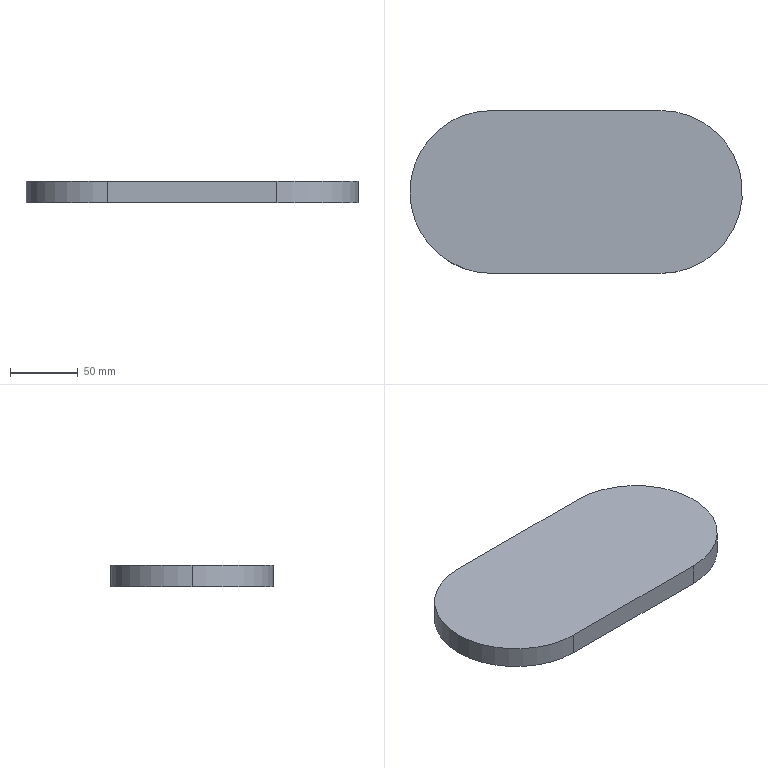Part | SolidWorks | features Extrusion 1 | 1 solid | 7 faces | box 245 x 120 x 16 mm | volume 420956 mm3 | plane 4 | cylinder 3 | commonest cylinder face diameters 120 x3
STEP:
#1=CARTESIAN_POINT('',(-122.5,0.,16.));
#2=VERTEX_POINT('',#1);
#3=CARTESIAN_POINT('',(-62.5,-60.,16.));
#4=VERTEX_POINT('',#3);
#5=CARTESIAN_POINT('',(-62.5,0.,16.));
#6=DIRECTION('',(0.,0.,1.));
#7=DIRECTION('',(1.,0.,0.));
#8=AXIS2_PLACEMENT_3D('',#5,#6,#7);
#9=CIRCLE('',#8,60.);
#10=EDGE_CURVE('',#2,#4,#9,.T.);
#11=ORIENTED_EDGE('',*,*,#10,.F.);
#12=CARTESIAN_POINT('',(-122.5,0.,0.));
#13=VERTEX_POINT('',#12);
#14=CARTESIAN_POINT('',(-122.5,0.,16.));
#15=DIRECTION('',(0.,0.,-1.));
#16=VECTOR('',#15,1000.);
#17=LINE('',#14,#16);
#18=EDGE_CURVE('',#2,#13,#17,.T.);
#19=ORIENTED_EDGE('',*,*,#18,.T.);
#20=CARTESIAN_POINT('',(-62.5,-60.,0.));
#21=VERTEX_POINT('',#20);
#22=CARTESIAN_POINT('',(-62.5,0.,0.));
#23=DIRECTION('',(0.,0.,1.));
#24=DIRECTION('',(1.,0.,0.));
#25=AXIS2_PLACEMENT_3D('',#22,#23,#24);
#26=CIRCLE('',#25,60.);
#27=EDGE_CURVE('',#13,#21,#26,.T.);
#28=ORIENTED_EDGE('',*,*,#27,.T.);
#29=CARTESIAN_POINT('',(-62.5,-60.,16.));
#30=DIRECTION('',(0.,0.,-1.));
#31=VECTOR('',#30,1000.);
#32=LINE('',#29,#31);
#33=EDGE_CURVE('',#4,#21,#32,.T.);
#34=ORIENTED_EDGE('',*,*,#33,.F.);
#35=EDGE_LOOP('',(#11,#19,#28,#34));
#36=FACE_OUTER_BOUND('',#35,.T.);
#37=CARTESIAN_POINT('',(-62.5,0.,16.));
#38=DIRECTION('',(0.,0.,-1.));
#39=DIRECTION('',(-1.,0.,0.));
#40=AXIS2_PLACEMENT_3D('',#37,#38,#39);
#41=CYLINDRICAL_SURFACE('',#40,60.);
#42=ADVANCED_FACE('',(#36),#41,.T.);
#43=ORIENTED_EDGE('',*,*,#18,.F.);
#44=CARTESIAN_POINT('',(-62.5,60.,16.));
#45=VERTEX_POINT('',#44);
#46=CARTESIAN_POINT('',(-62.5,0.,16.));
#47=DIRECTION('',(0.,0.,1.));
#48=DIRECTION('',(1.,0.,0.));
#49=AXIS2_PLACEMENT_3D('',#46,#47,#48);
#50=CIRCLE('',#49,60.);
#51=EDGE_CURVE('',#45,#2,#50,.T.);
#52=ORIENTED_EDGE('',*,*,#51,.F.);
#53=CARTESIAN_POINT('',(-62.5,60.,0.));
#54=VERTEX_POINT('',#53);
#55=CARTESIAN_POINT('',(-62.5,60.,16.));
#56=DIRECTION('',(0.,0.,-1.));
#57=VECTOR('',#56,1000.);
#58=LINE('',#55,#57);
#59=EDGE_CURVE('',#45,#54,#58,.T.);
#60=ORIENTED_EDGE('',*,*,#59,.T.);
#61=CARTESIAN_POINT('',(-62.5,0.,0.));
#62=DIRECTION('',(0.,0.,1.));
#63=DIRECTION('',(1.,0.,0.));
#64=AXIS2_PLACEMENT_3D('',#61,#62,#63);
#65=CIRCLE('',#64,60.);
#66=EDGE_CURVE('',#54,#13,#65,.T.);
#67=ORIENTED_EDGE('',*,*,#66,.T.);
#68=EDGE_LOOP('',(#43,#52,#60,#67));
#69=FACE_OUTER_BOUND('',#68,.T.);
#70=CARTESIAN_POINT('',(-62.5,0.,16.));
#71=DIRECTION('',(0.,0.,-1.));
#72=DIRECTION('',(-1.,0.,0.));
#73=AXIS2_PLACEMENT_3D('',#70,#71,#72);
#74=CYLINDRICAL_SURFACE('',#73,60.);
#75=ADVANCED_FACE('',(#69),#74,.T.);
#76=CARTESIAN_POINT('',(62.5,-60.,0.));
#77=VERTEX_POINT('',#76);
#78=CARTESIAN_POINT('',(-62.5,-60.,0.));
#79=DIRECTION('',(1.,0.,0.));
#80=VECTOR('',#79,1000.);
#81=LINE('',#78,#80);
#82=EDGE_CURVE('',#21,#77,#81,.T.);
#83=ORIENTED_EDGE('',*,*,#82,.T.);
#84=CARTESIAN_POINT('',(62.5,-60.,16.));
#85=VERTEX_POINT('',#84);
#86=CARTESIAN_POINT('',(62.5,-60.,16.));
#87=DIRECTION('',(0.,0.,-1.));
#88=VECTOR('',#87,1000.);
#89=LINE('',#86,#88);
#90=EDGE_CURVE('',#85,#77,#89,.T.);
#91=ORIENTED_EDGE('',*,*,#90,.F.);
#92=CARTESIAN_POINT('',(-62.5,-60.,16.));
#93=DIRECTION('',(1.,0.,0.));
#94=VECTOR('',#93,1000.);
#95=LINE('',#92,#94);
#96=EDGE_CURVE('',#4,#85,#95,.T.);
#97=ORIENTED_EDGE('',*,*,#96,.F.);
#98=ORIENTED_EDGE('',*,*,#33,.T.);
#99=EDGE_LOOP('',(#83,#91,#97,#98));
#100=FACE_OUTER_BOUND('',#99,.T.);
#101=CARTESIAN_POINT('',(-62.5,-60.,16.));
#102=DIRECTION('',(0.,1.,0.));
#103=DIRECTION('',(0.,0.,1.));
#104=AXIS2_PLACEMENT_3D('',#101,#102,#103);
#105=PLANE('',#104);
#106=ADVANCED_FACE('',(#100),#105,.F.);
#107=CARTESIAN_POINT('',(62.5,60.,0.));
#108=VERTEX_POINT('',#107);
#109=CARTESIAN_POINT('',(62.5,0.,0.));
#110=DIRECTION('',(0.,0.,1.));
#111=DIRECTION('',(1.,0.,0.));
#112=AXIS2_PLACEMENT_3D('',#109,#110,#111);
#113=CIRCLE('',#112,60.);
#114=EDGE_CURVE('',#77,#108,#113,.T.);
#115=ORIENTED_EDGE('',*,*,#114,.T.);
#116=CARTESIAN_POINT('',(62.5,60.,16.));
#117=VERTEX_POINT('',#116);
#118=CARTESIAN_POINT('',(62.5,60.,16.));
#119=DIRECTION('',(0.,0.,-1.));
#120=VECTOR('',#119,1000.);
#121=LINE('',#118,#120);
#122=EDGE_CURVE('',#117,#108,#121,.T.);
#123=ORIENTED_EDGE('',*,*,#122,.F.);
#124=CARTESIAN_POINT('',(62.5,0.,16.));
#125=DIRECTION('',(0.,0.,1.));
#126=DIRECTION('',(1.,0.,0.));
#127=AXIS2_PLACEMENT_3D('',#124,#125,#126);
#128=CIRCLE('',#127,60.);
#129=EDGE_CURVE('',#85,#117,#128,.T.);
#130=ORIENTED_EDGE('',*,*,#129,.F.);
#131=ORIENTED_EDGE('',*,*,#90,.T.);
#132=EDGE_LOOP('',(#115,#123,#130,#131));
#133=FACE_OUTER_BOUND('',#132,.T.);
#134=CARTESIAN_POINT('',(62.5,0.,16.));
#135=DIRECTION('',(0.,0.,-1.));
#136=DIRECTION('',(-1.,0.,0.));
#137=AXIS2_PLACEMENT_3D('',#134,#135,#136);
#138=CYLINDRICAL_SURFACE('',#137,60.);
#139=ADVANCED_FACE('',(#133),#138,.T.);
#140=CARTESIAN_POINT('',(-62.5,60.,0.));
#141=DIRECTION('',(-1.,0.,0.));
#142=VECTOR('',#141,1000.);
#143=LINE('',#140,#142);
#144=EDGE_CURVE('',#108,#54,#143,.T.);
#145=ORIENTED_EDGE('',*,*,#144,.T.);
#146=ORIENTED_EDGE('',*,*,#59,.F.);
#147=CARTESIAN_POINT('',(-62.5,60.,16.));
#148=DIRECTION('',(-1.,0.,0.));
#149=VECTOR('',#148,1000.);
#150=LINE('',#147,#149);
#151=EDGE_CURVE('',#117,#45,#150,.T.);
#152=ORIENTED_EDGE('',*,*,#151,.F.);
#153=ORIENTED_EDGE('',*,*,#122,.T.);
#154=EDGE_LOOP('',(#145,#146,#152,#153));
#155=FACE_OUTER_BOUND('',#154,.T.);
#156=CARTESIAN_POINT('',(-62.5,60.,16.));
#157=DIRECTION('',(0.,-1.,0.));
#158=DIRECTION('',(1.,0.,0.));
#159=AXIS2_PLACEMENT_3D('',#156,#157,#158);
#160=PLANE('',#159);
#161=ADVANCED_FACE('',(#155),#160,.F.);
#162=ORIENTED_EDGE('',*,*,#51,.T.);
#163=ORIENTED_EDGE('',*,*,#10,.T.);
#164=ORIENTED_EDGE('',*,*,#96,.T.);
#165=ORIENTED_EDGE('',*,*,#129,.T.);
#166=ORIENTED_EDGE('',*,*,#151,.T.);
#167=EDGE_LOOP('',(#162,#163,#164,#165,#166));
#168=FACE_OUTER_BOUND('',#167,.T.);
#169=CARTESIAN_POINT('',(-62.5,0.,16.));
#170=DIRECTION('',(0.,0.,1.));
#171=DIRECTION('',(1.,0.,0.));
#172=AXIS2_PLACEMENT_3D('',#169,#170,#171);
#173=PLANE('',#172);
#174=ADVANCED_FACE('',(#168),#173,.T.);
#175=ORIENTED_EDGE('',*,*,#66,.F.);
#176=ORIENTED_EDGE('',*,*,#144,.F.);
#177=ORIENTED_EDGE('',*,*,#114,.F.);
#178=ORIENTED_EDGE('',*,*,#82,.F.);
#179=ORIENTED_EDGE('',*,*,#27,.F.);
#180=EDGE_LOOP('',(#175,#176,#177,#178,#179));
#181=FACE_OUTER_BOUND('',#180,.T.);
#182=CARTESIAN_POINT('',(-62.5,0.,0.));
#183=DIRECTION('',(0.,0.,1.));
#184=DIRECTION('',(1.,0.,0.));
#185=AXIS2_PLACEMENT_3D('',#182,#183,#184);
#186=PLANE('',#185);
#187=ADVANCED_FACE('',(#181),#186,.F.);
#188=CLOSED_SHELL('',(#42,#75,#106,#139,#161,#174,#187));
#189=MANIFOLD_SOLID_BREP('',#188);
#190=CARTESIAN_POINT('',(0.,0.,0.));
#191=DIRECTION('',(0.,0.,1.));
#192=DIRECTION('',(1.,0.,0.));
#193=AXIS2_PLACEMENT_3D('',#190,#191,#192);
#194=(LENGTH_UNIT()NAMED_UNIT(*)SI_UNIT(.MILLI.,.METRE.));
#195=UNCERTAINTY_MEASURE_WITH_UNIT(LENGTH_MEASURE(0.00001),#194,'','');
#196=(NAMED_UNIT(*)PLANE_ANGLE_UNIT()SI_UNIT($,.RADIAN.));
#197=(NAMED_UNIT(*)SI_UNIT($,.STERADIAN.)SOLID_ANGLE_UNIT());
#198=(GEOMETRIC_REPRESENTATION_CONTEXT(3)GLOBAL_UNCERTAINTY_ASSIGNED_CONTEXT((#195))GLOBAL_UNIT_ASSIGNED_CONTEXT((#194,#196,#197))REPRESENTATION_CONTEXT('',''));
#199=ADVANCED_BREP_SHAPE_REPRESENTATION('',(#189,#193),#198);